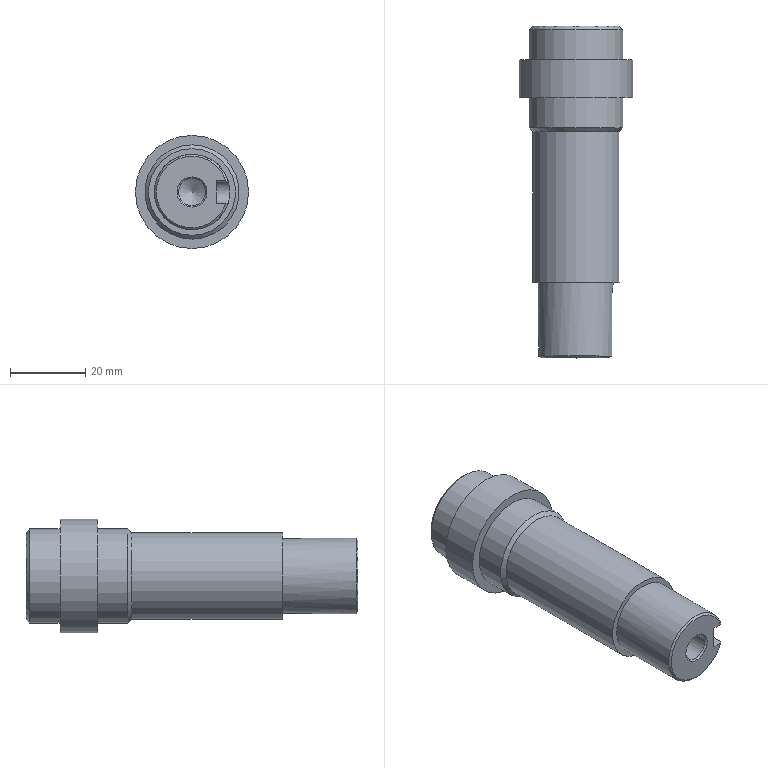Part | NX | features DATUM_CSYS 3, EXTRUDE 3, CHAMFER 2, SKETCH 2, FACE_BLEND 1, HOLE PACKAGE 1, SIMPLE HOLE 1, SWP104 1, SYMBOLIC_THREAD 1 | 1 solid | 20 faces | box 30 x 88 x 30 mm | volume 37691 mm3 | plane 8 | cylinder 7 | cone 5 | commonest cylinder face diameters 25 x2 6 x1 7.2 x1 20 x1 23 x1 30 x1
STEP:
#1=CARTESIAN_POINT('',(0.,79.,12.5));
#2=VERTEX_POINT('',#1);
#3=CARTESIAN_POINT('',(0.,79.,0.));
#4=DIRECTION('',(0.,1.,0.));
#5=DIRECTION('',(0.,0.,1.));
#6=AXIS2_PLACEMENT_3D('',#3,#4,#5);
#7=CIRCLE('',#6,12.5);
#8=EDGE_CURVE('',#2,#2,#7,.T.);
#9=ORIENTED_EDGE('',*,*,#8,.F.);
#10=EDGE_LOOP('',(#9));
#11=FACE_BOUND('',#10,.T.);
#12=CARTESIAN_POINT('',(0.,79.,15.));
#13=VERTEX_POINT('',#12);
#14=CARTESIAN_POINT('',(0.,79.,0.));
#15=DIRECTION('',(0.,1.,0.));
#16=DIRECTION('',(0.,0.,1.));
#17=AXIS2_PLACEMENT_3D('',#14,#15,#16);
#18=CIRCLE('',#17,15.);
#19=EDGE_CURVE('',#13,#13,#18,.T.);
#20=ORIENTED_EDGE('',*,*,#19,.T.);
#21=EDGE_LOOP('',(#20));
#22=FACE_BOUND('',#21,.T.);
#23=CARTESIAN_POINT('',(0.,79.,0.));
#24=DIRECTION('',(0.,1.,0.));
#25=DIRECTION('',(0.,0.,1.));
#26=AXIS2_PLACEMENT_3D('',#23,#24,#25);
#27=PLANE('',#26);
#28=ADVANCED_FACE('',(#11,#22),#27,.T.);
#29=ORIENTED_EDGE('',*,*,#19,.F.);
#30=EDGE_LOOP('',(#29));
#31=FACE_BOUND('',#30,.T.);
#32=CARTESIAN_POINT('',(0.,69.,15.));
#33=VERTEX_POINT('',#32);
#34=CARTESIAN_POINT('',(0.,69.,0.));
#35=DIRECTION('',(0.,1.,0.));
#36=DIRECTION('',(0.,0.,1.));
#37=AXIS2_PLACEMENT_3D('',#34,#35,#36);
#38=CIRCLE('',#37,15.);
#39=EDGE_CURVE('',#33,#33,#38,.T.);
#40=ORIENTED_EDGE('',*,*,#39,.T.);
#41=EDGE_LOOP('',(#40));
#42=FACE_BOUND('',#41,.T.);
#43=CARTESIAN_POINT('',(0.,0.,0.));
#44=DIRECTION('',(0.,1.,0.));
#45=DIRECTION('',(0.,0.,1.));
#46=AXIS2_PLACEMENT_3D('',#43,#44,#45);
#47=CYLINDRICAL_SURFACE('',#46,15.);
#48=ADVANCED_FACE('',(#31,#42),#47,.T.);
#49=ORIENTED_EDGE('',*,*,#39,.F.);
#50=EDGE_LOOP('',(#49));
#51=FACE_BOUND('',#50,.T.);
#52=CARTESIAN_POINT('',(0.,69.,12.5));
#53=VERTEX_POINT('',#52);
#54=CARTESIAN_POINT('',(0.,69.,0.));
#55=DIRECTION('',(0.,1.,0.));
#56=DIRECTION('',(0.,0.,1.));
#57=AXIS2_PLACEMENT_3D('',#54,#55,#56);
#58=CIRCLE('',#57,12.5);
#59=EDGE_CURVE('',#53,#53,#58,.T.);
#60=ORIENTED_EDGE('',*,*,#59,.T.);
#61=EDGE_LOOP('',(#60));
#62=FACE_BOUND('',#61,.T.);
#63=CARTESIAN_POINT('',(0.,69.,12.5));
#64=DIRECTION('',(0.,1.,0.));
#65=DIRECTION('',(0.,0.,1.));
#66=AXIS2_PLACEMENT_3D('',#63,#64,#65);
#67=PLANE('',#66);
#68=ADVANCED_FACE('',(#51,#62),#67,.F.);
#69=CARTESIAN_POINT('',(0.,61.,12.5));
#70=VERTEX_POINT('',#69);
#71=CARTESIAN_POINT('',(0.,61.,0.));
#72=DIRECTION('',(0.,1.,0.));
#73=DIRECTION('',(0.,0.,1.));
#74=AXIS2_PLACEMENT_3D('',#71,#72,#73);
#75=CIRCLE('',#74,12.5);
#76=EDGE_CURVE('',#70,#70,#75,.T.);
#77=ORIENTED_EDGE('',*,*,#76,.T.);
#78=EDGE_LOOP('',(#77));
#79=FACE_BOUND('',#78,.T.);
#80=ORIENTED_EDGE('',*,*,#59,.F.);
#81=EDGE_LOOP('',(#80));
#82=FACE_BOUND('',#81,.T.);
#83=CARTESIAN_POINT('',(0.,0.,0.));
#84=DIRECTION('',(0.,1.,0.));
#85=DIRECTION('',(0.,0.,1.));
#86=AXIS2_PLACEMENT_3D('',#83,#84,#85);
#87=CYLINDRICAL_SURFACE('',#86,12.5);
#88=ADVANCED_FACE('',(#79,#82),#87,.T.);
#89=CARTESIAN_POINT('',(0.,87.,12.5));
#90=VERTEX_POINT('',#89);
#91=CARTESIAN_POINT('',(0.,87.,0.));
#92=DIRECTION('',(0.,1.,0.));
#93=DIRECTION('',(0.,0.,1.));
#94=AXIS2_PLACEMENT_3D('',#91,#92,#93);
#95=CIRCLE('',#94,12.5);
#96=EDGE_CURVE('',#90,#90,#95,.F.);
#97=ORIENTED_EDGE('',*,*,#96,.T.);
#98=EDGE_LOOP('',(#97));
#99=FACE_BOUND('',#98,.T.);
#100=ORIENTED_EDGE('',*,*,#8,.T.);
#101=EDGE_LOOP('',(#100));
#102=FACE_BOUND('',#101,.T.);
#103=CARTESIAN_POINT('',(0.,88.,0.));
#104=DIRECTION('',(0.,-1.,0.));
#105=DIRECTION('',(0.,0.,-1.));
#106=AXIS2_PLACEMENT_3D('',#103,#104,#105);
#107=CYLINDRICAL_SURFACE('',#106,12.5);
#108=ADVANCED_FACE('',(#99,#102),#107,.T.);
#109=CARTESIAN_POINT('',(0.,88.,11.5));
#110=VERTEX_POINT('',#109);
#111=CARTESIAN_POINT('',(0.,88.,0.));
#112=DIRECTION('',(0.,1.,0.));
#113=DIRECTION('',(0.,0.,1.));
#114=AXIS2_PLACEMENT_3D('',#111,#112,#113);
#115=CIRCLE('',#114,11.5);
#116=EDGE_CURVE('',#110,#110,#115,.T.);
#117=ORIENTED_EDGE('',*,*,#116,.T.);
#118=EDGE_LOOP('',(#117));
#119=FACE_BOUND('',#118,.T.);
#120=CARTESIAN_POINT('',(0.,88.,0.));
#121=DIRECTION('',(0.,1.,0.));
#122=DIRECTION('',(0.,0.,1.));
#123=AXIS2_PLACEMENT_3D('',#120,#121,#122);
#124=PLANE('',#123);
#125=ADVANCED_FACE('',(#119),#124,.T.);
#126=CARTESIAN_POINT('',(0.,20.,11.5));
#127=VERTEX_POINT('',#126);
#128=CARTESIAN_POINT('',(0.,20.,0.));
#129=DIRECTION('',(0.,1.,0.));
#130=DIRECTION('',(0.,0.,1.));
#131=AXIS2_PLACEMENT_3D('',#128,#129,#130);
#132=CIRCLE('',#131,11.5);
#133=EDGE_CURVE('',#127,#127,#132,.T.);
#134=ORIENTED_EDGE('',*,*,#133,.F.);
#135=EDGE_LOOP('',(#134));
#136=FACE_BOUND('',#135,.T.);
#137=CARTESIAN_POINT('',(10.,20.,0.));
#138=VERTEX_POINT('',#137);
#139=CARTESIAN_POINT('',(0.,20.,0.));
#140=DIRECTION('',(0.,1.,0.));
#141=DIRECTION('',(0.,0.,1.));
#142=AXIS2_PLACEMENT_3D('',#139,#140,#141);
#143=CIRCLE('',#142,10.);
#144=EDGE_CURVE('',#138,#138,#143,.T.);
#145=ORIENTED_EDGE('',*,*,#144,.T.);
#146=EDGE_LOOP('',(#145));
#147=FACE_BOUND('',#146,.T.);
#148=CARTESIAN_POINT('',(0.,20.,0.));
#149=DIRECTION('',(0.,1.,0.));
#150=DIRECTION('',(0.,0.,1.));
#151=AXIS2_PLACEMENT_3D('',#148,#149,#150);
#152=PLANE('',#151);
#153=ADVANCED_FACE('',(#136,#147),#152,.F.);
#154=ORIENTED_EDGE('',*,*,#133,.T.);
#155=EDGE_LOOP('',(#154));
#156=FACE_BOUND('',#155,.T.);
#157=CARTESIAN_POINT('',(0.,60.,11.5));
#158=VERTEX_POINT('',#157);
#159=CARTESIAN_POINT('',(0.,60.,0.));
#160=DIRECTION('',(0.,1.,0.));
#161=DIRECTION('',(0.,0.,1.));
#162=AXIS2_PLACEMENT_3D('',#159,#160,#161);
#163=CIRCLE('',#162,11.5);
#164=EDGE_CURVE('',#158,#158,#163,.T.);
#165=ORIENTED_EDGE('',*,*,#164,.F.);
#166=EDGE_LOOP('',(#165));
#167=FACE_BOUND('',#166,.T.);
#168=CARTESIAN_POINT('',(0.,20.,0.));
#169=DIRECTION('',(0.,1.,0.));
#170=DIRECTION('',(0.,0.,1.));
#171=AXIS2_PLACEMENT_3D('',#168,#169,#170);
#172=CYLINDRICAL_SURFACE('',#171,11.5);
#173=ADVANCED_FACE('',(#156,#167),#172,.T.);
#174=CARTESIAN_POINT('',(0.,15.,3.6));
#175=VERTEX_POINT('',#174);
#176=CARTESIAN_POINT('',(0.,15.,0.));
#177=DIRECTION('',(0.,1.,0.));
#178=DIRECTION('',(0.,0.,1.));
#179=AXIS2_PLACEMENT_3D('',#176,#177,#178);
#180=CIRCLE('',#179,3.6);
#181=EDGE_CURVE('',#175,#175,#180,.F.);
#182=ORIENTED_EDGE('',*,*,#181,.T.);
#183=EDGE_LOOP('',(#182));
#184=FACE_BOUND('',#183,.T.);
#185=CARTESIAN_POINT('',(0.,17.163,0.));
#186=VERTEX_POINT('',#185);
#187=VERTEX_LOOP('',#186);
#188=FACE_BOUND('',#187,.T.);
#189=CARTESIAN_POINT('',(0.,15.,0.));
#190=DIRECTION('',(0.,-1.,0.));
#191=DIRECTION('',(0.,0.,-1.));
#192=AXIS2_PLACEMENT_3D('',#189,#190,#191);
#193=CONICAL_SURFACE('',#192,3.6,1.03);
#194=ADVANCED_FACE('',(#184,#188),#193,.F.);
#195=CARTESIAN_POINT('',(0.,0.4,3.6));
#196=VERTEX_POINT('',#195);
#197=CARTESIAN_POINT('',(0.,0.4,0.));
#198=DIRECTION('',(0.,1.,0.));
#199=DIRECTION('',(0.,0.,1.));
#200=AXIS2_PLACEMENT_3D('',#197,#198,#199);
#201=CIRCLE('',#200,3.6);
#202=EDGE_CURVE('',#196,#196,#201,.F.);
#203=ORIENTED_EDGE('',*,*,#202,.T.);
#204=EDGE_LOOP('',(#203));
#205=FACE_BOUND('',#204,.T.);
#206=ORIENTED_EDGE('',*,*,#181,.F.);
#207=EDGE_LOOP('',(#206));
#208=FACE_BOUND('',#207,.T.);
#209=CARTESIAN_POINT('',(0.,0.,0.));
#210=DIRECTION('',(0.,1.,0.));
#211=DIRECTION('',(0.,0.,1.));
#212=AXIS2_PLACEMENT_3D('',#209,#210,#211);
#213=CYLINDRICAL_SURFACE('',#212,3.6);
#214=ADVANCED_FACE('',(#205,#208),#213,.F.);
#215=ORIENTED_EDGE('',*,*,#202,.F.);
#216=EDGE_LOOP('',(#215));
#217=FACE_BOUND('',#216,.T.);
#218=CARTESIAN_POINT('',(0.,0.,4.));
#219=VERTEX_POINT('',#218);
#220=CARTESIAN_POINT('',(0.,0.,0.));
#221=DIRECTION('',(0.,1.,0.));
#222=DIRECTION('',(0.,0.,1.));
#223=AXIS2_PLACEMENT_3D('',#220,#221,#222);
#224=CIRCLE('',#223,4.);
#225=EDGE_CURVE('',#219,#219,#224,.T.);
#226=ORIENTED_EDGE('',*,*,#225,.F.);
#227=EDGE_LOOP('',(#226));
#228=FACE_BOUND('',#227,.T.);
#229=CARTESIAN_POINT('',(0.,0.,0.));
#230=DIRECTION('',(0.,-1.,0.));
#231=DIRECTION('',(0.,0.,-1.));
#232=AXIS2_PLACEMENT_3D('',#229,#230,#231);
#233=CONICAL_SURFACE('',#232,4.,0.7854);
#234=ADVANCED_FACE('',(#217,#228),#233,.F.);
#235=CARTESIAN_POINT('',(6.5,0.,-3.));
#236=VERTEX_POINT('',#235);
#237=CARTESIAN_POINT('',(6.5,17.,-3.));
#238=VERTEX_POINT('',#237);
#239=CARTESIAN_POINT('',(6.5,20.,-3.));
#240=DIRECTION('',(0.,-1.,0.));
#241=VECTOR('',#240,1000.);
#242=LINE('',#239,#241);
#243=EDGE_CURVE('',#236,#238,#242,.F.);
#244=ORIENTED_EDGE('',*,*,#243,.T.);
#245=CARTESIAN_POINT('',(6.5,17.,3.));
#246=VERTEX_POINT('',#245);
#247=CARTESIAN_POINT('',(6.5,17.,0.));
#248=DIRECTION('',(-1.,0.,0.));
#249=DIRECTION('',(0.,0.,1.));
#250=AXIS2_PLACEMENT_3D('',#247,#248,#249);
#251=CIRCLE('',#250,3.);
#252=EDGE_CURVE('',#238,#246,#251,.F.);
#253=ORIENTED_EDGE('',*,*,#252,.T.);
#254=CARTESIAN_POINT('',(6.5,0.,3.));
#255=VERTEX_POINT('',#254);
#256=CARTESIAN_POINT('',(6.5,20.,3.));
#257=DIRECTION('',(0.,-1.,0.));
#258=VECTOR('',#257,1000.);
#259=LINE('',#256,#258);
#260=EDGE_CURVE('',#255,#246,#259,.F.);
#261=ORIENTED_EDGE('',*,*,#260,.F.);
#262=CARTESIAN_POINT('',(6.5,0.,3.));
#263=DIRECTION('',(0.,0.,-1.));
#264=VECTOR('',#263,1000.);
#265=LINE('',#262,#264);
#266=EDGE_CURVE('',#255,#236,#265,.T.);
#267=ORIENTED_EDGE('',*,*,#266,.T.);
#268=EDGE_LOOP('',(#244,#253,#261,#267));
#269=FACE_BOUND('',#268,.T.);
#270=CARTESIAN_POINT('',(6.5,20.,3.));
#271=DIRECTION('',(-1.,0.,0.));
#272=DIRECTION('',(0.,0.,1.));
#273=AXIS2_PLACEMENT_3D('',#270,#271,#272);
#274=PLANE('',#273);
#275=ADVANCED_FACE('',(#269),#274,.F.);
#276=CARTESIAN_POINT('',(9.539,0.5,3.));
#277=VERTEX_POINT('',#276);
#278=CARTESIAN_POINT('',(9.539,17.,3.));
#279=VERTEX_POINT('',#278);
#280=CARTESIAN_POINT('',(9.539,0.,3.));
#281=DIRECTION('',(0.,1.,0.));
#282=VECTOR('',#281,1000.);
#283=LINE('',#280,#282);
#284=EDGE_CURVE('',#277,#279,#283,.T.);
#285=ORIENTED_EDGE('',*,*,#284,.F.);
#286=CARTESIAN_POINT('',(9.014,0.,3.));
#287=VERTEX_POINT('',#286);
#288=CARTESIAN_POINT('',(9.539,0.5,3.));
#289=CARTESIAN_POINT('',(9.364,0.3331,3.));
#290=CARTESIAN_POINT('',(9.189,0.1664,3.));
#291=CARTESIAN_POINT('',(9.014,0.,3.));
#292=B_SPLINE_CURVE_WITH_KNOTS('',3,(#288,#289,#290,#291),.UNSPECIFIED.,.F.,.F.,(4,4),(0.,0.0007254),.UNSPECIFIED.);
#293=EDGE_CURVE('',#277,#287,#292,.T.);
#294=ORIENTED_EDGE('',*,*,#293,.T.);
#295=CARTESIAN_POINT('',(18.5,0.,3.));
#296=DIRECTION('',(-1.,0.,0.));
#297=VECTOR('',#296,1000.);
#298=LINE('',#295,#297);
#299=EDGE_CURVE('',#287,#255,#298,.T.);
#300=ORIENTED_EDGE('',*,*,#299,.T.);
#301=ORIENTED_EDGE('',*,*,#260,.T.);
#302=CARTESIAN_POINT('',(18.5,17.,3.));
#303=DIRECTION('',(1.,0.,0.));
#304=VECTOR('',#303,1000.);
#305=LINE('',#302,#304);
#306=EDGE_CURVE('',#246,#279,#305,.T.);
#307=ORIENTED_EDGE('',*,*,#306,.T.);
#308=EDGE_LOOP('',(#285,#294,#300,#301,#307));
#309=FACE_BOUND('',#308,.T.);
#310=CARTESIAN_POINT('',(18.5,20.,3.));
#311=DIRECTION('',(0.,0.,1.));
#312=DIRECTION('',(1.,0.,0.));
#313=AXIS2_PLACEMENT_3D('',#310,#311,#312);
#314=PLANE('',#313);
#315=ADVANCED_FACE('',(#309),#314,.F.);
#316=ORIENTED_EDGE('',*,*,#225,.T.);
#317=EDGE_LOOP('',(#316));
#318=FACE_BOUND('',#317,.T.);
#319=ORIENTED_EDGE('',*,*,#299,.F.);
#320=CARTESIAN_POINT('',(9.014,0.,-3.));
#321=VERTEX_POINT('',#320);
#322=CARTESIAN_POINT('',(0.,0.,0.));
#323=DIRECTION('',(0.,1.,0.));
#324=DIRECTION('',(0.,0.,1.));
#325=AXIS2_PLACEMENT_3D('',#322,#323,#324);
#326=CIRCLE('',#325,9.5);
#327=EDGE_CURVE('',#287,#321,#326,.F.);
#328=ORIENTED_EDGE('',*,*,#327,.T.);
#329=CARTESIAN_POINT('',(6.5,0.,-3.));
#330=DIRECTION('',(1.,0.,0.));
#331=VECTOR('',#330,1000.);
#332=LINE('',#329,#331);
#333=EDGE_CURVE('',#236,#321,#332,.T.);
#334=ORIENTED_EDGE('',*,*,#333,.F.);
#335=ORIENTED_EDGE('',*,*,#266,.F.);
#336=EDGE_LOOP('',(#319,#328,#334,#335));
#337=FACE_BOUND('',#336,.T.);
#338=CARTESIAN_POINT('',(0.,0.,0.));
#339=DIRECTION('',(0.,1.,0.));
#340=DIRECTION('',(0.,0.,1.));
#341=AXIS2_PLACEMENT_3D('',#338,#339,#340);
#342=PLANE('',#341);
#343=ADVANCED_FACE('',(#318,#337),#342,.F.);
#344=ORIENTED_EDGE('',*,*,#333,.T.);
#345=CARTESIAN_POINT('',(9.539,0.5,-3.));
#346=VERTEX_POINT('',#345);
#347=CARTESIAN_POINT('',(9.014,0.,-3.));
#348=CARTESIAN_POINT('',(9.189,0.1664,-3.));
#349=CARTESIAN_POINT('',(9.364,0.3331,-3.));
#350=CARTESIAN_POINT('',(9.539,0.5,-3.));
#351=B_SPLINE_CURVE_WITH_KNOTS('',3,(#347,#348,#349,#350),.UNSPECIFIED.,.F.,.F.,(4,4),(0.,0.0007254),.UNSPECIFIED.);
#352=EDGE_CURVE('',#321,#346,#351,.T.);
#353=ORIENTED_EDGE('',*,*,#352,.T.);
#354=CARTESIAN_POINT('',(9.539,17.,-3.));
#355=VERTEX_POINT('',#354);
#356=CARTESIAN_POINT('',(9.539,0.,-3.));
#357=DIRECTION('',(0.,1.,0.));
#358=VECTOR('',#357,1000.);
#359=LINE('',#356,#358);
#360=EDGE_CURVE('',#355,#346,#359,.F.);
#361=ORIENTED_EDGE('',*,*,#360,.F.);
#362=CARTESIAN_POINT('',(6.5,17.,-3.));
#363=DIRECTION('',(1.,0.,0.));
#364=VECTOR('',#363,1000.);
#365=LINE('',#362,#364);
#366=EDGE_CURVE('',#355,#238,#365,.F.);
#367=ORIENTED_EDGE('',*,*,#366,.T.);
#368=ORIENTED_EDGE('',*,*,#243,.F.);
#369=EDGE_LOOP('',(#344,#353,#361,#367,#368));
#370=FACE_BOUND('',#369,.T.);
#371=CARTESIAN_POINT('',(6.5,20.,-3.));
#372=DIRECTION('',(0.,0.,-1.));
#373=DIRECTION('',(-1.,0.,0.));
#374=AXIS2_PLACEMENT_3D('',#371,#372,#373);
#375=PLANE('',#374);
#376=ADVANCED_FACE('',(#370),#375,.F.);
#377=CARTESIAN_POINT('',(10.,20.,0.));
#378=CARTESIAN_POINT('',(10.,20.,-0.7973));
#379=CARTESIAN_POINT('',(9.775,19.345,-2.343));
#380=CARTESIAN_POINT('',(9.539,17.797,-3.));
#381=CARTESIAN_POINT('',(9.539,17.,-3.));
#382=B_SPLINE_CURVE_WITH_KNOTS('',3,(#377,#378,#379,#380,#381),.UNSPECIFIED.,.F.,.F.,(4,1,4),(0.004714,0.007071,0.009428),.UNSPECIFIED.);
#383=EDGE_CURVE('',#355,#138,#382,.F.);
#384=ORIENTED_EDGE('',*,*,#383,.T.);
#385=CARTESIAN_POINT('',(9.539,17.,3.));
#386=CARTESIAN_POINT('',(9.539,17.797,3.));
#387=CARTESIAN_POINT('',(9.775,19.343,2.345));
#388=CARTESIAN_POINT('',(10.,20.,0.7973));
#389=CARTESIAN_POINT('',(10.,20.,0.));
#390=B_SPLINE_CURVE_WITH_KNOTS('',3,(#385,#386,#387,#388,#389),.UNSPECIFIED.,.F.,.F.,(4,1,4),(0.,0.002357,0.004714),.UNSPECIFIED.);
#391=EDGE_CURVE('',#138,#279,#390,.F.);
#392=ORIENTED_EDGE('',*,*,#391,.T.);
#393=ORIENTED_EDGE('',*,*,#306,.F.);
#394=ORIENTED_EDGE('',*,*,#252,.F.);
#395=ORIENTED_EDGE('',*,*,#366,.F.);
#396=EDGE_LOOP('',(#384,#392,#393,#394,#395));
#397=FACE_BOUND('',#396,.T.);
#398=CARTESIAN_POINT('',(6.5,17.,0.));
#399=DIRECTION('',(1.,0.,0.));
#400=DIRECTION('',(0.,1.,0.));
#401=AXIS2_PLACEMENT_3D('',#398,#399,#400);
#402=CYLINDRICAL_SURFACE('',#401,3.);
#403=ADVANCED_FACE('',(#397),#402,.F.);
#404=ORIENTED_EDGE('',*,*,#360,.T.);
#405=CARTESIAN_POINT('',(0.,0.5,0.));
#406=DIRECTION('',(0.,1.,0.));
#407=DIRECTION('',(0.,0.,1.));
#408=AXIS2_PLACEMENT_3D('',#405,#406,#407);
#409=CIRCLE('',#408,10.);
#410=EDGE_CURVE('',#346,#277,#409,.T.);
#411=ORIENTED_EDGE('',*,*,#410,.T.);
#412=ORIENTED_EDGE('',*,*,#284,.T.);
#413=ORIENTED_EDGE('',*,*,#391,.F.);
#414=ORIENTED_EDGE('',*,*,#144,.F.);
#415=ORIENTED_EDGE('',*,*,#383,.F.);
#416=EDGE_LOOP('',(#404,#411,#412,#413,#414,#415));
#417=FACE_BOUND('',#416,.T.);
#418=CARTESIAN_POINT('',(0.,0.,0.));
#419=DIRECTION('',(0.,1.,0.));
#420=DIRECTION('',(0.,0.,1.));
#421=AXIS2_PLACEMENT_3D('',#418,#419,#420);
#422=CYLINDRICAL_SURFACE('',#421,10.);
#423=ADVANCED_FACE('',(#417),#422,.T.);
#424=ORIENTED_EDGE('',*,*,#96,.F.);
#425=EDGE_LOOP('',(#424));
#426=FACE_BOUND('',#425,.T.);
#427=ORIENTED_EDGE('',*,*,#116,.F.);
#428=EDGE_LOOP('',(#427));
#429=FACE_BOUND('',#428,.T.);
#430=CARTESIAN_POINT('',(0.,88.,0.));
#431=DIRECTION('',(0.,-1.,0.));
#432=DIRECTION('',(0.,0.,-1.));
#433=AXIS2_PLACEMENT_3D('',#430,#431,#432);
#434=CONICAL_SURFACE('',#433,11.5,0.7854);
#435=ADVANCED_FACE('',(#426,#429),#434,.T.);
#436=ORIENTED_EDGE('',*,*,#164,.T.);
#437=EDGE_LOOP('',(#436));
#438=FACE_BOUND('',#437,.T.);
#439=ORIENTED_EDGE('',*,*,#76,.F.);
#440=EDGE_LOOP('',(#439));
#441=FACE_BOUND('',#440,.T.);
#442=CARTESIAN_POINT('',(0.,61.,0.));
#443=DIRECTION('',(0.,1.,0.));
#444=DIRECTION('',(0.,0.,1.));
#445=AXIS2_PLACEMENT_3D('',#442,#443,#444);
#446=CONICAL_SURFACE('',#445,12.5,0.7854);
#447=ADVANCED_FACE('',(#438,#441),#446,.T.);
#448=ORIENTED_EDGE('',*,*,#352,.F.);
#449=ORIENTED_EDGE('',*,*,#327,.F.);
#450=ORIENTED_EDGE('',*,*,#293,.F.);
#451=ORIENTED_EDGE('',*,*,#410,.F.);
#452=EDGE_LOOP('',(#448,#449,#450,#451));
#453=FACE_BOUND('',#452,.T.);
#454=CARTESIAN_POINT('',(0.,0.5,0.));
#455=DIRECTION('',(0.,1.,0.));
#456=DIRECTION('',(0.,0.,1.));
#457=AXIS2_PLACEMENT_3D('',#454,#455,#456);
#458=CONICAL_SURFACE('',#457,10.,0.7854);
#459=ADVANCED_FACE('',(#453),#458,.T.);
#460=CLOSED_SHELL('',(#28,#48,#68,#88,#108,#125,#153,#173,#194,#214,#234,#275,#315,#343,#376,#403,#423,#435,#447,#459));
#461=MANIFOLD_SOLID_BREP('',#460);
#462=(LENGTH_UNIT()NAMED_UNIT(*)SI_UNIT(.MILLI.,.METRE.));
#463=UNCERTAINTY_MEASURE_WITH_UNIT(LENGTH_MEASURE(0.0508),#462,'','');
#464=(NAMED_UNIT(*)PLANE_ANGLE_UNIT()SI_UNIT($,.RADIAN.));
#465=(NAMED_UNIT(*)SI_UNIT($,.STERADIAN.)SOLID_ANGLE_UNIT());
#466=(GEOMETRIC_REPRESENTATION_CONTEXT(3)GLOBAL_UNCERTAINTY_ASSIGNED_CONTEXT((#463))GLOBAL_UNIT_ASSIGNED_CONTEXT((#462,#464,#465))REPRESENTATION_CONTEXT('',''));
#467=ADVANCED_BREP_SHAPE_REPRESENTATION('',(#461),#466);